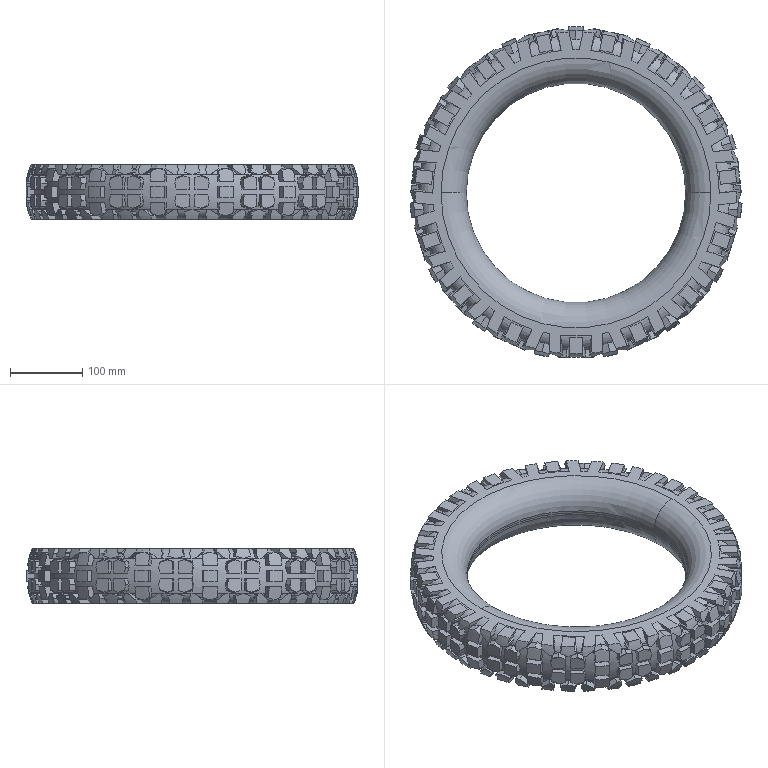Part | SolidWorks | features BaseBody 1 | 1 solid | 2682 faces | box 461.727 x 459.625 x 76.2 mm | volume 2396758 mm3 | plane 2449 | torus 225 | cylinder 8 | commonest cylinder face diameters 304.8 x4 314.8 x4